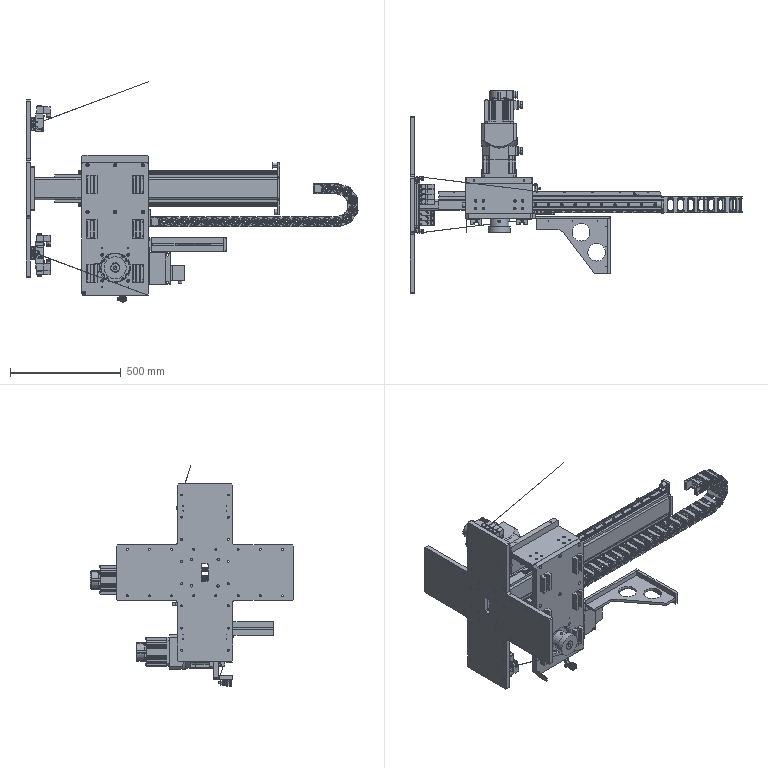Part | SolidWorks | features InContextFeatHolder 40, ReferencePattern 26, LocalLPattern 4, LocalCirPattern 1, MirrorCompFeat 1 | 86 solids | 15819 faces | volume 39375353 mm3 | cylinder 7856 | plane 6835 | cone 864 | spline 124 | torus 114 | sphere 26 | commonest cylinder face diameters 2 x1001 1 x768 4 x380 20.12 x240 5 x237 11 x236